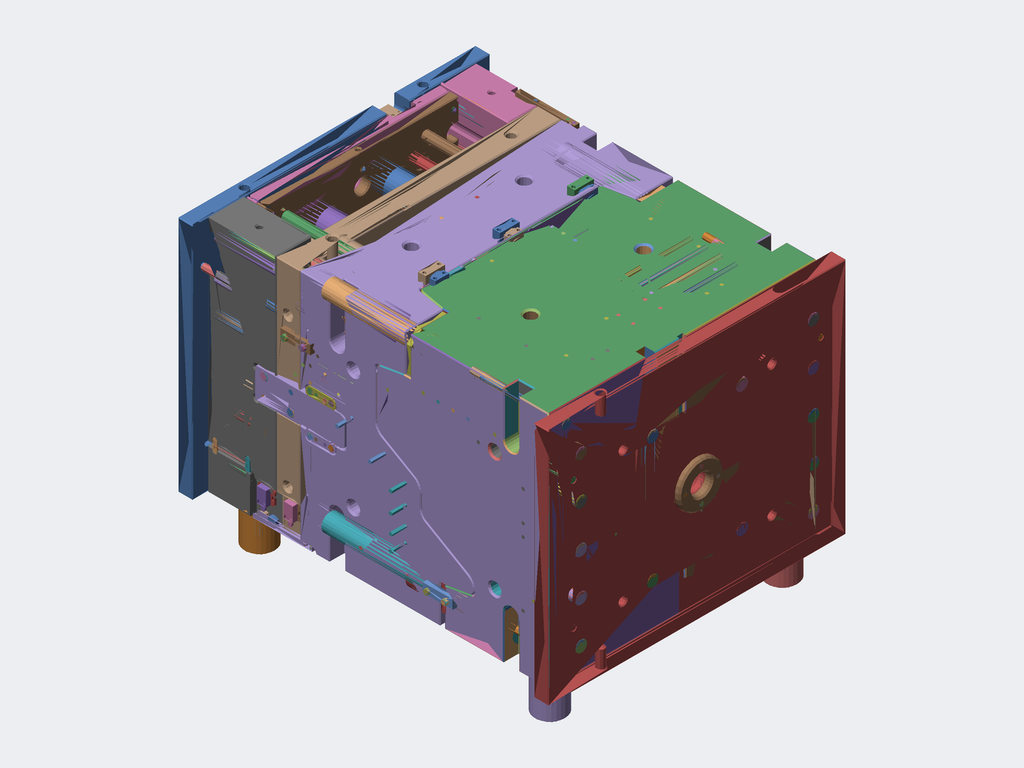Assembly | STEP file | 277 different items | 1042 placed
Parts list (item | name | quantity | parent item | size | volume):
1 | 1 | x1 | in A2 | 550 x 62 x 62 mm | 1011386 mm3
2 | 1-1 | x1 | in A2 | 150 x 62 x 62 mm | 225988 mm3
3 | 35-TOE-IN(B35) | x2 | in A2 | 34 x 20 x 20 mm | 6255 mm3
4 | 35-TOE-out(BIM35) | x2 | in A2 | 83 x 35 x 30.398 mm | 24144 mm3
5 | BOLT(all)(M8X60) | x4 | in A2 | 60 x 13 x 13 mm | 3384 mm3
6 | BRACKET-none | x1 | in A2 | 45 x 39 x 52 mm | 53167 mm3
7 | Bolt M6(M6[10]) | x2 | in A2 | 16 x 10 x 10 mm | 667.21 mm3
8 | DOWEL DISC(DOWEL DISC(Φ29.5×10)) | x1 | in A2 | 10 x 29.5 x 29.5 mm | 4862 mm3
9 | DOWEL PIN(DOWEL PIN(Φ15×33)) | x1 | in A2 | 33 x 15 x 15 mm | 5582 mm3
10 | Disc Pad | x2 | in A2 | 9.5 x 39 x 39 mm | 6734 mm3
11 | INSULATION DISC | x1 | in A2 | 12 x 29.2 x 219.2 mm | 11077 mm3
12 | LOCK PIN(LOCK PIN(Φ10×30)) | x1 | in A2 | 30 x 10 x 10 mm | 2277 mm3
13 | M8_NL23(L=15) | x4 | in A2 | 22.4 x 12.98 x 12.98 mm | 1605 mm3
14 | NL23,33(NL23_SR21(D4-D8)) | x1 | in A2 | 35 x 56 x 56 mm | 57560 mm3
15 | Nozzle Body(02) | x1 | in A2 | 497 x 60 x 60 mm | 469077 mm3
16 | Nozzle Body-2(02) | x1 | in A2 | 97 x 60 x 60 mm | 109750 mm3
17 | Snap Ring_Bala35 | x2 | in A2 | 1.75 x 36 x 34.918 mm | 197.431 mm3
18 | Tube Heater_Bala35_toe | x1 | in A2 | 219 x 96.332 x 96.332 mm | 165765 mm3
19 | Tube Heater_Bala35_toe-1 | x1 | in A2 | 259.756 x 47 x 47 mm | 158264 mm3
20 | Tube Heater_Bala35_toe-2 | x1 | in A2 | 69 x 90.077 x 102.033 mm | 51909 mm3
21 | V802 | x1 | in A2 | 45 x 88 x 289.568 mm | 783132 mm3
22 | solid 1 | x2 | in A2 | 110 x 70 x 149 mm | 483474 mm3
23 | solid 10 | x2 | in A2 | 935 x 17 x 17 mm | 106657 mm3
24 | solid 11 | x2 | in A2 | 580 x 17 x 17 mm | 66508 mm3
25 | solid 12 | x2 | in A2 | 11.557 x 13.074 x 13.001 mm | 528.422 mm3
26 | solid 125 | x2 | in A2 | 25 x 12 x 18 mm | 4663 mm3
27 | solid 126 | x2 | in A2 | 10 x 10 x 23.5 mm | 895.066 mm3
28 | solid 127 | x2 | in A2 | 11 x 11 x 27 mm | 1102 mm3
29 | solid 128 | x2 | in A2 | 10 x 10 x 26.5 mm | 979.889 mm3
30 | solid 129 | x2 | in A2 | 11 x 11 x 30 mm | 1201 mm3
31 | solid 13 | x2 | in A2 | 12.797 x 15.596 x 14.273 mm | 763.699 mm3
32 | solid 130 | x1 | in A2 | 198 x 17 x 14 mm | 37768 mm3
33 | solid 131 | x2 | in A2 | 10 x 10 x 26.5 mm | 979.889 mm3
34 | solid 132 | x2 | in A2 | 11 x 11 x 30 mm | 1201 mm3
35 | solid 133 | x2 | in A2 | 11 x 11 x 27 mm | 1102 mm3
36 | solid 134 | x2 | in A2 | 10 x 10 x 23.5 mm | 895.066 mm3
37 | solid 135 | x1 | in A2 | 198 x 17 x 14 mm | 37768 mm3
38 | solid 136 | x2 | in A2 | 25 x 12 x 18 mm | 4663 mm3
39 | solid 137 | x2 | in A2 | 30 x 16 x 70 mm | 24653 mm3
40 | solid 138 | x2 | in A2 | 20 x 15 x 15 mm | 3534 mm3
41 | solid 139 | x2 | in A2 | 12 x 358 x 176 mm | 59139 mm3
42 | solid 14 | x2 | in A2 | 230 x 60 x 60 mm | 648335 mm3
43 | solid 140 | x1 | in A2 | 614 x 415 x 490 mm | 485763 mm3
44 | solid 141 | x1 | in A2 | - | 250615157 mm3
45 | solid 142 | x1 | in A2 | 80 x 900 x 800 mm | 51885032 mm3
46 | solid 143 | x1 | in A2 | 501 x 18 x 18 mm | 57793 mm3
47 | solid 144 | x6 | in A2 | 260 x 30 x 30 mm | 86664 mm3
48 | solid 145 | x6 | in A2 | 270.5 x 32 x 32 mm | 104702 mm3
49 | solid 146 | x5 | in A2 | 195.123 x 11 x 13 mm | 10096 mm3
50 | solid 147 | x14 | in A2 | 95 x 36 x 36 mm | 52905 mm3
51 | solid 148 | x14 | in A2 | 107.5 x 39 x 39 mm | 61848 mm3
52 | solid 149 | x6 | in A2 | 204 x 46 x 46 mm | 139116 mm3
53 | solid 15 | x8 | in A2 | 67.5 x 16 x 16 mm | 6227 mm3
54 | solid 150 | x2 | in A2 | 52.5 x 10 x 10 mm | 1715 mm3
55 | solid 151 | x2 | in A2 | 59.59 x 11 x 11 mm | 2247 mm3
56 | solid 152 | x10 | in A2 | 27.5 x 10 x 10 mm | 1008 mm3
57 | solid 153 | x2 | in A2 | 36.597 x 11 x 11 mm | 1608 mm3
58 | solid 154 | x1 | in A2 | 652.487 x 245.59 x 387.851 mm | 665208 mm3
59 | solid 155 | x1 | in A2 | 238.099 x 35 x 343.322 mm | 1118074 mm3
60 | solid 156 | x1 | in A2 | 247.177 x 50 x 457.681 mm | 843242 mm3
61 | solid 157 | x1 | in A2 | 2.637 x 0.8538 x 0.6297 mm | 0.1595 mm3
62 | solid 158 | x2 | in A2 | 136 x 80 x 80 mm | 299080 mm3
63 | solid 159 | x2 | in A2 | 195.5 x 32 x 32 mm | 76192 mm3
64 | solid 16 | x1 | in A2 | 30 x 650 x 800 mm | 13444333 mm3
65 | solid 160 | x2 | in A2 | 185 x 30 x 30 mm | 63102 mm3
66 | solid 161 | x2 | in A2 | 650 x 60 x 60 mm | 1835397 mm3
67 | solid 162 | x1 | in A2 | 300 x 45 x 100 mm | 1292632 mm3
68 | solid 163 | x1 | in A2 | 300 x 45 x 100 mm | 1292632 mm3
69 | solid 164 | x4 | in A2 | 16 x 75 x 16 mm | 15080 mm3
70 | solid 165 | x4 | in A2 | 20 x 71.5 x 20 mm | 10497 mm3
71 | solid 166 | x8 | in A2 | 12 x 70 x 12 mm | 7917 mm3
72 | solid 167 | x10 | in A2 | 18 x 65 x 18 mm | 8589 mm3
73 | solid 168 | x2 | in A2 | 26 x 83.5 x 26 mm | 21746 mm3
74 | solid 169 | x2 | in A2 | 100 x 45 x 30 mm | 102688 mm3
75 | solid 17 | x1 | in A2 | 35 x 650 x 800 mm | 15784723 mm3
76 | solid 170 | x2 | in A2 | 24 x 75 x 24 mm | 17852 mm3
77 | solid 171 | x2 | in A2 | 26 x 83.5 x 26 mm | 21746 mm3
78 | solid 172 | x2 | in A2 | 24 x 75 x 24 mm | 17852 mm3
79 | solid 173 | x4 | in A2 | 20 x 71.5 x 20 mm | 10497 mm3
80 | solid 174 | x4 | in A2 | 18 x 65 x 18 mm | 8589 mm3
81 | solid 175 | x2 | in A2 | 100 x 45 x 30 mm | 102688 mm3
82 | solid 176 | x4 | in A2 | 12 x 900 x 12 mm | 101788 mm3
83 | solid 177 | x4 | in A2 | 12 x 1000 x 12 mm | 113097 mm3
84 | solid 178 | x4 | in A2 | 80.521 x 100 x 23.74 mm | 76082 mm3
85 | solid 179 | x10 | in A2 | 11.612 x 10 x 23.374 mm | 866.792 mm3
86 | solid 18 | x2 | in A2 | 13 x 13 x 45 mm | 2786 mm3
87 | solid 180 | x10 | in A2 | 12.22 x 11 x 26.693 mm | 1068 mm3
88 | solid 181 | x2 | in A2 | 80.521 x 100 x 23.74 mm | 64518 mm3
89 | solid 182 | x1 | in A2 | 80.521 x 100 x 23.74 mm | 76082 mm3
90 | solid 183 | x1 | in A2 | 652.487 x 245.59 x 387.851 mm | 667269 mm3
91 | solid 184 | x2 | in A2 | 489.684 x 12 x 12 mm | 55371 mm3
92 | solid 185 | x6 | in A2 | 539.477 x 12.005 x 12.001 mm | 58014 mm3
93 | solid 186 | x2 | in A2 | 371.47 x 12.005 x 12 mm | 41921 mm3
94 | solid 187 | x8 | in A2 | 439.33 x 12.005 x 12.001 mm | 46615 mm3
95 | solid 188 | x2 | in A2 | 435.109 x 12 x 12 mm | 48874 mm3
96 | solid 189 | x2 | in A2 | 489.594 x 12 x 12 mm | 55372 mm3
97 | solid 19 | x2 | in A2 | 14 x 14 x 49.5 mm | 3399 mm3
98 | solid 190 | x2 | in A2 | 724.85 x 12 x 12.001 mm | 81515 mm3
99 | solid 191 | x12 | in A2 | 469.808 x 10.006 x 10.001 mm | 35280 mm3
100 | solid 192 | x1 | in A2 | 855 x 12 x 12 mm | 96698 mm3
101 | solid 193 | x4 | in A2 | 134.268 x 10 x 10 mm | 10442 mm3
102 | solid 194 | x1 | in A2 | 652.487 x 245.902 x 387.851 mm | 656196 mm3
103 | solid 195 | x1 | in A2 | 175.156 x 75 x 109.18 mm | 273394 mm3
104 | solid 196 | x2 | in A2 | 84 x 20 x 20 mm | 26155 mm3
105 | solid 197 | x2 | in A2 | 84 x 20 x 20 mm | 26155 mm3
106 | solid 198 | x4 | in A2 | 15 x 120 x 120 mm | 132037 mm3
107 | solid 199 | x8 | in A2 | 85 x 10 x 10 mm | 6676 mm3
108 | solid 2 | x2 | in A2 | 56.962 x 48 x 38.66 mm | 28035 mm3
109 | solid 20 | x2 | in A2 | 40 x 30 x 30 mm | 30325 mm3
110 | solid 200 | x8 | in A2 | 88 x 18 x 18 mm | 9169 mm3
111 | solid 201 | x6 | in A2 | 42.525 x 20 x 69.579 mm | 10496 mm3
112 | solid 202 | x2 | in A2 | 138 x 446 x 305 mm | 147324 mm3
113 | solid 203 | x8 | in A2 | 10 x 60 x 90 mm | 51612 mm3
114 | solid 204 | x8 | in A2 | 82.5 x 16 x 16 mm | 7406 mm3
115 | solid 205 | x24 | in A2 | 26 x 26 x 68.5 mm | 17929 mm3
116 | solid 206 | x2 | in A2 | 180 x 44.5 x 45 mm | 267303 mm3
117 | solid 207 | x24 | in A2 | 24 x 24 x 60 mm | 14836 mm3
118 | solid 208 | x2 | in A2 | 705 x 476 x 374 mm | 3235310 mm3
119 | solid 209 | x2 | in A2 | 35 x 13 x 13 mm | 2283 mm3
120 | solid 21 | x1 | in A2 | 15 x 124 x 12.156 mm | 19013 mm3
121 | solid 210 | x2 | in A2 | 150 x 80 x 80 mm | 329867 mm3
122 | solid 211 | x2 | in A2 | 39.5 x 14 x 14 mm | 2762 mm3
123 | solid 212 | x2 | in A2 | 470 x 481 x 467.5 mm | 693577 mm3
124 | solid 213 | x2 | in A2 | 263.363 x 10.007 x 10 mm | 18382 mm3
125 | solid 214 | x16 | in A2 | 16 x 16 x 70 mm | 14074 mm3
126 | solid 215 | x4 | in A2 | 20 x 20 x 76.5 mm | 11160 mm3
127 | solid 216 | x4 | in A2 | 16 x 16 x 110 mm | 22117 mm3
128 | solid 217 | x4 | in A2 | 18 x 18 x 70 mm | 9155 mm3
129 | solid 218 | x6 | in A2 | 16 x 16 x 90 mm | 18096 mm3
130 | solid 219 | x2 | in A2 | 120 x 20 x 20 mm | 37465 mm3
131 | solid 22 | x2 | in A2 | 1260 x 12 x 12 mm | 142503 mm3
132 | solid 220 | x4 | in A2 | 220 x 66 x 66 mm | 626724 mm3
133 | solid 221 | x4 | in A2 | 24 x 24 x 80 mm | 18857 mm3
134 | solid 222 | x4 | in A2 | 10 x 10 x 19.5 mm | 781.969 mm3
135 | solid 223 | x2 | in A2 | 120 x 20 x 20 mm | 37465 mm3
136 | solid 224 | x4 | in A2 | 11 x 11 x 23 mm | 968.93 mm3
137 | solid 225 | x1 | in A2 | 140 x 226.5 x 45 mm | 911767 mm3
138 | solid 226 | x2 | in A2 | 9.737 x 7 x 9.737 mm | 407.483 mm3
139 | solid 227 | x4 | in A2 | 26 x 26 x 88.5 mm | 23018 mm3
140 | solid 228 | x4 | in A2 | 50 x 80 x 80 mm | 107474 mm3
141 | solid 229 | x2 | in A2 | 180 x 44.5 x 45 mm | 267303 mm3
142 | solid 23 | x1 | in A2 | 81.042 x 12 x 90.722 mm | 14374 mm3
143 | solid 230 | x2 | in A2 | 96.9 x 70 x 101.844 mm | 150796 mm3
144 | solid 231 | x1 | in A2 | 140 x 44.5 x 45 mm | 196703 mm3
145 | solid 232 | x2 | in A2 | 221.793 x 70 x 90 mm | 892401 mm3
146 | solid 233 | x4 | in A2 | 26 x 26 x 108.5 mm | 28107 mm3
147 | solid 234 | x2 | in A2 | 34.555 x 24 x 45.236 mm | 13572 mm3
148 | solid 235 | x2 | in A2 | 280 x 40 x 50 mm | 488862 mm3
149 | solid 236 | x4 | in A2 | 24 x 24 x 100 mm | 22879 mm3
150 | solid 237 | x3 | in A2 | 52 x 46 x 19 mm | 33444 mm3
151 | solid 238 | x3 | in A2 | 25 x 65 x 27 mm | 26512 mm3
152 | solid 239 | x8 | in A2 | 31 x 11 x 11 mm | 1234 mm3
153 | solid 24 | x2 | in A2 | 1160 x 12 x 12 mm | 131193 mm3
154 | solid 240 | x1 | in A2 | 24.594 x 40 x 40 mm | 25514 mm3
155 | solid 241 | x2 | in A2 | 65 x 30 x 116 mm | 157735 mm3
156 | solid 242 | x2 | in A2 | 91.603 x 70 x 58.66 mm | 66082 mm3
157 | solid 243 | x2 | in A2 | 45 x 66 x 106 mm | 203588 mm3
158 | solid 244 | x2 | in A2 | 80.636 x 23 x 57.712 mm | 28005 mm3
159 | solid 245 | x4 | in A2 | 10 x 80 x 120 mm | 92082 mm3
160 | solid 246 | x3 | in A2 | 25 x 65 x 27 mm | 26512 mm3
161 | solid 247 | x3 | in A2 | 52 x 46 x 19 mm | 33444 mm3
162 | solid 248 | x1 | in A2 | 81.775 x 66 x 117.55 mm | 328210 mm3
163 | solid 249 | x2 | in A2 | 39 x 13 x 13 mm | 2484 mm3
164 | solid 25 | x1 | in A2 | 160.634 x 12 x 91.227 mm | 21883 mm3
165 | solid 250 | x2 | in A2 | 65 x 30 x 116 mm | 157735 mm3
166 | solid 251 | x2 | in A2 | 44.094 x 14 x 14 mm | 3108 mm3
167 | solid 252 | x6 | in A2 | 373.765 x 8.5 x 8.5 mm | 4948 mm3
168 | solid 253 | x2 | in A2 | 520 x 60 x 60 mm | 1467831 mm3
169 | solid 254 | x8 | in A2 | 63 x 18 x 18 mm | 6793 mm3
170 | solid 255 | x1 | in A2 | 322.109 x 11 x 13 mm | 16427 mm3
171 | solid 256 | x8 | in A2 | 57.5 x 16 x 16 mm | 5442 mm3
172 | solid 257 | x1 | in A2 | 687.344 x 385 x 800 mm | 676592 mm3
173 | solid 258 | x2 | in A2 | 325.5 x 32 x 32 mm | 125610 mm3
174 | solid 259 | x2 | in A2 | 315 x 30 x 30 mm | 103942 mm3
175 | solid 26 | x2 | in A2 | 17.629 x 21.043 x 6.038 mm | 691.957 mm3
176 | solid 260 | x1 | in A2 | 570 x 292.75 x 800 mm | 1618507 mm3
177 | solid 261 | x2 | in A2 | 533.706 x 13 x 13 mm | 27276 mm3
178 | solid 262 | x1 | in A2 | 175.156 x 75 x 109.18 mm | 273394 mm3
179 | solid 263 | x2 | in A2 | 9.737 x 7 x 9.737 mm | 407.483 mm3
180 | solid 264 | x1 | in A2 | 570 x 292.75 x 800 mm | 1618507 mm3
181 | solid 265 | x1 | in A2 | 687.344 x 385 x 800 mm | 676593 mm3
182 | solid 266 | x1 | in A2 | 140 x 44.5 x 45 mm | 196703 mm3
183 | solid 267 | x1 | in A2 | 140 x 226.5 x 45 mm | 911767 mm3
184 | solid 268 | x1 | in A2 | 652.466 x 245.902 x 388.968 mm | 650950 mm3
185 | solid 269 | x1 | in A2 | 10 x 40 x 90 mm | 33612 mm3
186 | solid 27 | x2 | in A2 | 18.904 x 20.052 x 6.503 mm | 764.337 mm3
187 | solid 270 | x22 | in A2 | 995 x 10 x 10 mm | 78147 mm3
188 | solid 271 | x1 | in A2 | 19.849 x 36 x 36 mm | 16717 mm3
189 | solid 272 | x1 | in A2 | 24.594 x 40 x 40 mm | 25466 mm3
190 | solid 273 | x1 | in A2 | 81.775 x 66 x 117.55 mm | 328215 mm3
191 | solid 274 | x1 | in A2 | 33.29 x 11.457 x 16.18 mm | 703.754 mm3
192 | solid 275 | x1 | in A2 | 652.466 x 245.902 x 388.968 mm | 649456 mm3
193 | solid 276 | x1 | in A2 | 34.494 x 28.911 x 22.331 mm | 948.282 mm3
194 | solid 277 | x1 | in A2 | 67.648 x 83.054 x 185.27 mm | 23432 mm3
195 | solid 278 | x1 | in A2 | 60 x 80 x 80 mm | 335456 mm3
196 | solid 279 | x1 | in A2 | 652.466 x 245.902 x 388.968 mm | 651328 mm3
197 | solid 28 | x1 | in A2 | 35.828 x 104 x 11.998 mm | 37179 mm3
198 | solid 29 | x2 | in A2 | 120 x 45 x 50 mm | 204594 mm3
199 | solid 3 | x60 | in A2 | 17.678 x 10 x 22.986 mm | 866.792 mm3
200 | solid 30 | x2 | in A2 | 120 x 45 x 50 mm | 204595 mm3
201 | solid 31 | x6 | in A2 | 230 x 80 x 80 mm | 1153880 mm3
202 | solid 32 | x6 | in A2 | 730 x 17 x 15 mm | 83352 mm3
203 | solid 33 | x2 | in A2 | 670 x 17 x 15 mm | 76566 mm3
204 | solid 34 | x2 | in A2 | 640 x 17 x 15 mm | 73173 mm3
205 | solid 35 | x2 | in A2 | 580 x 15 x 13 mm | 46226 mm3
206 | solid 36 | x2 | in A2 | 940 x 15 x 13 mm | 74501 mm3
207 | solid 37 | x2 | in A2 | 700 x 17 x 15 mm | 79959 mm3
208 | solid 38 | x2 | in A2 | 890 x 15 x 13 mm | 70574 mm3
209 | solid 39 | x1 | in A2 | 901 x 18 x 18 mm | 103032 mm3
210 | solid 4 | x60 | in A2 | 19.428 x 11 x 25.651 mm | 1068 mm3
211 | solid 40 | x2 | in A2 | 820 x 17 x 15 mm | 93531 mm3
212 | solid 41 | x2 | in A2 | 405 x 15 x 13 mm | 32482 mm3
213 | solid 42 | x2 | in A2 | 670 x 15 x 13 mm | 53295 mm3
214 | solid 43 | x2 | in A2 | 955 x 17 x 15 mm | 108799 mm3
215 | solid 44 | x2 | in A2 | 825 x 15 x 13 mm | 65469 mm3
216 | solid 45 | x2 | in A2 | 905 x 17 x 15 mm | 103144 mm3
217 | solid 46 | x2 | in A2 | 370 x 15 x 13 mm | 29733 mm3
218 | solid 47 | x2 | in A2 | 610 x 17 x 15 mm | 69781 mm3
219 | solid 48 | x2 | in A2 | 585 x 15 x 13 mm | 46619 mm3
220 | solid 49 | x2 | in A2 | 445 x 15 x 13 mm | 35624 mm3
221 | solid 5 | x1 | in A2 | 238.099 x 35 x 343.322 mm | 1118038 mm3
222 | solid 50 | x2 | in A2 | 800 x 17 x 15 mm | 91269 mm3
223 | solid 51 | x2 | in A2 | 855 x 17 x 15 mm | 97489 mm3
224 | solid 52 | x4 | in A2 | 265 x 30 x 30 mm | 88234 mm3
225 | solid 53 | x12 | in A2 | 325 x 36 x 36 mm | 156954 mm3
226 | solid 54 | x12 | in A2 | 337.5 x 39 x 39 mm | 183962 mm3
227 | solid 55 | x2 | in A2 | 406 x 36 x 36 mm | 287307 mm3
228 | solid 56 | x1 | in A2 | 230 x 120 x 800 mm | 20287508 mm3
229 | solid 57 | x1 | in A2 | 230 x 120 x 800 mm | 20301168 mm3
230 | solid 58 | x21 | in A2 | 15 x 5 x 45 mm | 2940 mm3
231 | solid 59 | x21 | in A2 | 11.5 x 15 x 11.5 mm | 365.141 mm3
232 | solid 6 | x2 | in A2 | 20.1 x 20.1 x 20.1 mm | 4252 mm3
233 | solid 60 | x6 | in A2 | 49 x 56 x 6 mm | 15004 mm3
234 | solid 61 | x4 | in A2 | 70 x 30 x 16 mm | 24653 mm3
235 | solid 62 | x15 | in A2 | 15 x 30 x 30 mm | 4037 mm3
236 | solid 63 | x15 | in A2 | 65 x 24 x 24 mm | 15841 mm3
237 | solid 64 | x15 | in A2 | 73.5 x 26 x 26 mm | 19201 mm3
238 | solid 65 | x12 | in A2 | 77 x 18 x 18 mm | 8123 mm3
239 | solid 66 | x12 | in A2 | 71.5 x 16 x 16 mm | 6542 mm3
240 | solid 67 | x4 | in A2 | 54 x 45 x 45 mm | 77782 mm3
241 | solid 68 | x4 | in A2 | 54 x 45 x 45 mm | 77782 mm3
242 | solid 69 | x2 | in A2 | 54 x 35 x 35 mm | 44135 mm3
243 | solid 7 | x1 | in A2 | 652.487 x 245.59 x 387.851 mm | 665466 mm3
244 | solid 70 | x2 | in A2 | 54 x 35 x 35 mm | 44135 mm3
245 | solid 71 | x1 | in A2 | 50 x 1000 x 800 mm | 37110850 mm3
246 | solid 72 | x2 | in A2 | 736 x 36 x 36 mm | 520571 mm3
247 | solid 73 | x4 | in A2 | 300 x 35 x 35 mm | 211977 mm3
248 | solid 74 | x4 | in A2 | 55 x 48 x 48 mm | 41563 mm3
249 | solid 75 | x4 | in A2 | 275.5 x 32 x 32 mm | 106603 mm3
250 | solid 76 | x2 | in A2 | 170 x 20 x 20 mm | 53173 mm3
251 | solid 77 | x4 | in A2 | 32 x 32 x 165.5 mm | 64789 mm3
252 | solid 78 | x2 | in A2 | 170 x 20 x 20 mm | 53173 mm3
253 | solid 79 | x4 | in A2 | 30 x 30 x 155 mm | 53677 mm3
254 | solid 8 | x1 | in A2 | 19.849 x 36 x 36 mm | 16739 mm3
255 | solid 80 | x2 | in A2 | 100 x 100 x 120 mm | 885185 mm3
256 | solid 81 | x2 | in A2 | 100 x 100 x 120 mm | 885185 mm3
257 | solid 82 | x4 | in A2 | 16 x 42.5 x 16 mm | 4264 mm3
258 | solid 83 | x4 | in A2 | 18 x 48 x 18 mm | 5406 mm3
259 | solid 84 | x4 | in A2 | 100 x 15 x 30 mm | 42149 mm3
260 | solid 85 | x4 | in A2 | 16 x 42.5 x 16 mm | 4264 mm3
261 | solid 86 | x4 | in A2 | 18 x 48 x 18 mm | 5406 mm3
262 | solid 87 | x4 | in A2 | 40 x 13 x 13 mm | 2534 mm3
263 | solid 88 | x4 | in A2 | 44.5 x 14 x 14 mm | 3080 mm3
264 | solid 89 | x1 | in A2 | 50 x 1000 x 800 mm | 38736605 mm3
265 | solid 9 | x1 | in A2 | 652.487 x 245.59 x 387.851 mm | 665205 mm3
266 | solid 90 | x2 | in A2 | 540 x 80 x 90 mm | 3073364 mm3
267 | solid 91 | x1 | in A2 | 25 x 150 x 150 mm | 329738 mm3
268 | solid 92 | x2 | in A2 | 5 x 30 x 5 mm | 589.049 mm3
269 | solid 93 | x2 | in A2 | 26.72 x 10 x 46.022 mm | 3002 mm3
270 | solid 94 | x2 | in A2 | 5 x 35 x 5 mm | 687.223 mm3
271 | solid 95 | x2 | in A2 | 29.477 x 10 x 49.99 mm | 3007 mm3
272 | solid 96 | x1 | in A2 | 247.177 x 50 x 457.681 mm | 845709 mm3
273 | solid 97 | x2 | in A2 | 140.241 x 15 x 428.298 mm | 50261 mm3
274 | solid 98 | x2 | in A2 | 74.766 x 17 x 208.871 mm | 24808 mm3
275 | 平头螺丝(M6) | x1 | in A2 | 12 x 12 x 12 mm | 449.452 mm3
276 | Part 1^V802 | x1 | in A2 | 9.5 x 94.25 x 254.4 mm | 39991 mm3
277 | Part 1^V802DS | x1 | in A2 | 9.5 x 94.25 x 254.4 mm | 39991 mm3